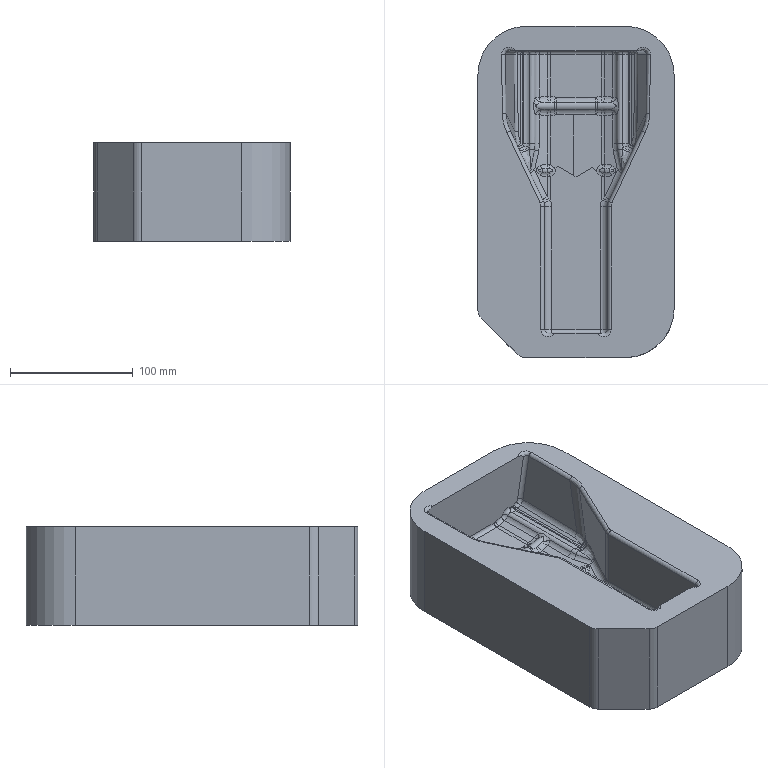NC program | NX | posted with a generic post | part box 160 x 270 x 80 mm
Lines 1 to 1083 of 159324:
N10 G17 G21 G94 G90
(CAVITY_MILL , TOOL : D25R5)
N12 T00 M6
N14 G54
N16 G17 G0 G90 X-4.895 Y47.373 S1200 M3
N18 G43 Z10. H0
N20 Z3.
N22 G94 G3 X5.06 Y53.831 Z-0.349 R11.25 F2000.
N24 G1 X10.121 Y64.585
N26 X-10.121
N28 X0. Y43.077
N30 X5.06 Y53.831
N32 X11.847 Y50.638
N34 X18.788 Y65.388
N36 X18.876 Y72.085
N38 X-18.876
N40 X-18.788 Y65.388
N42 X0. Y25.462
N44 X11.847 Y50.638
N46 X18.633 Y47.444
N48 X25.857 Y62.796
N50 G3 X26.278 Y64.583 R4.349
N52 G1 X26.476 Y79.585
N54 X-26.476
N56 X-26.278 Y64.583
N58 G3 X-25.852 Y62.787 R4.349
N60 G1 X0. Y7.848
N62 X18.633 Y47.444
N64 X25.419 Y44.251
N66 X32.639 Y59.595
N68 G3 X33.777 Y64.468 R11.849
N70 G1 X34.076 Y87.085
N72 X-34.076
N74 X-33.777 Y64.468
N76 G3 X-32.633 Y59.582 R11.849
N78 G1 X-5.628 Y2.194
N80 G2 X-2.469 Y-11.942 R33.204
N82 G1 Y-87.086
N84 X2.469
N86 Y-11.942
N88 G2 X5.628 Y2.194 R33.204
N90 G1 X25.419 Y44.251
N92 X32.205 Y41.058
N94 X39.419 Y56.387
N96 G3 X41.276 Y64.358 R19.349
N98 G1 X41.676 Y94.585
N100 X-41.676
N102 X-41.276 Y64.358
N104 G3 X-39.415 Y56.379 R19.349
N106 G1 X-12.415 Y-0.999
N108 G2 X-9.969 Y-11.942 R25.704
N110 G1 Y-94.587
N112 X9.969 Y-94.585
N114 Y-11.942
N116 G2 X12.415 Y-0.999 R25.704
N118 G1 X32.205 Y41.058
N120 X38.991 Y37.864
N122 X46.198 Y53.179
N124 G3 X48.775 Y64.25 R26.849
N126 G1 X49.309 Y104.589
N128 X49.247
N130 X49.191
N132 Y104.55
N134 X47.872 Y103.604
N136 X47.332 Y103.228
N138 X47.06 Y103.046
N140 X46.479 Y102.68
N142 X46.167 Y102.501
N144 X45.993 Y102.408
N146 X45.763 Y102.296
N148 X45.227 Y102.108
N150 X45.083 Y102.087
N152 X44.99 Y102.085
N154 X-44.954
N156 X-45.063 Y102.086
N158 X-45.2 Y102.103
N160 X-45.801 Y102.314
N162 X-46.028 Y102.426
N164 X-46.229 Y102.535
N166 X-46.478 Y102.68
N168 X-47.059 Y103.046
N170 X-48.197 Y103.837
N172 X-49.195 Y104.571
N174 Y104.589
N176 X-49.256
N178 X-49.309
N180 X-48.775 Y64.25
N182 G3 X-46.198 Y53.179 R26.849
N184 G1 X-19.201 Y-4.192
N186 G2 X-17.469 Y-11.942 R18.204
N188 G1 Y-104.589
N190 X-17.372
N192 X-16.937 Y-104.259
N194 X-15.66 Y-103.33
N196 X-15.469 Y-103.199
N198 X-15.241 Y-103.046
N200 X-14.694 Y-102.697
N202 X-14.143 Y-102.387
N204 X-13.757 Y-102.212
N206 X-13.432 Y-102.087
N208 X13.319 Y-102.085
N210 X13.515 Y-102.13
N212 X13.759 Y-102.213
N214 X13.961 Y-102.299
N216 X14.929 Y-102.843
N218 X15.241 Y-103.046
N220 X15.469 Y-103.199
N222 X17.19 Y-104.451
N224 X17.367 Y-104.589
N226 X17.469
N228 Y-11.942
N230 G2 X19.201 Y-4.192 R18.204
N232 G1 X38.991 Y37.864
N234 X27.681 Y43.187
N236 Z2.651
N238 G0 Z10.
N240 X-5.254 Y48.135
N242 Z2.651
N244 G3 X4.702 Y54.592 Z-0.699 R11.25
N246 G1 X9.404 Y64.585
N248 X-9.404
N250 X0. Y44.6
N252 X4.702 Y54.592
N254 X11.488 Y51.399
N256 X18.141 Y65.537
N258 X18.228 Y72.085
N260 X-18.228
N262 X-18.141 Y65.537
N264 X0. Y26.985
N266 X11.488 Y51.399
N268 X18.275 Y48.206
N270 X25.263 Y63.057
N272 G3 X25.63 Y64.621 R3.797
N274 G1 X25.828 Y79.585
N276 X-25.828
N278 X-25.63 Y64.646
N280 G3 X-25.257 Y63.044 R3.881
N282 G1 X0. Y9.37
N284 X18.275 Y48.206
N286 X25.061 Y45.012
N288 X32.047 Y59.858
N290 G3 X33.129 Y64.512 R11.297
N292 G1 X33.427 Y87.085
N294 X-33.427
N296 X-33.129 Y64.542
N298 G3 X-32.041 Y59.847 R11.381
N300 G1 X-5.045 Y2.478
N302 G2 X-1.821 Y-11.942 R33.852
N304 G1 Y-87.086
N306 X1.821
N308 Y-11.942
N310 G2 X5.036 Y2.457 R33.852
N312 G1 X25.061 Y45.012
N314 X31.847 Y41.819
N316 X38.827 Y56.653
N318 G3 X40.628 Y64.405 R18.797
N320 G1 X41.027 Y94.585
N322 X-41.027
N324 X-40.629 Y64.439
N326 G3 X-38.826 Y56.651 R18.881
N328 G1 X-11.831 Y-0.717
N330 G2 X-9.321 Y-11.942 R26.352
N332 G1 Y-94.587
N334 X9.321 Y-94.585
N336 Y-11.942
N338 G2 X11.823 Y-0.733 R26.352
N340 G1 X31.847 Y41.819
N342 X38.633 Y38.626
N344 X45.611 Y53.455
N346 G3 X48.127 Y64.3 R26.297
N348 G1 X48.654 Y104.097
N350 X48.56
N352 X47.872 Y103.604
N354 X47.332 Y103.228
N356 X47.06 Y103.046
N358 X46.479 Y102.68
N360 X46.167 Y102.501
N362 X45.993 Y102.408
N364 X45.763 Y102.296
N366 X45.227 Y102.108
N368 X45.083 Y102.087
N370 X44.99 Y102.085
N372 X-44.954
N374 X-45.063 Y102.086
N376 X-45.2 Y102.103
N378 X-45.801 Y102.314
N380 X-46.028 Y102.426
N382 X-46.229 Y102.535
N384 X-46.478 Y102.68
N386 X-47.059 Y103.046
N388 X-48.197 Y103.837
N390 X-48.551 Y104.097
N392 X-48.654
N394 X-48.128 Y64.336
N396 G3 X-45.611 Y53.455 R26.381
N398 G1 X-18.618 Y-3.908
N400 G2 X-16.821 Y-11.942 R18.852
N402 G1 Y-104.097
N404 X-16.714
N406 X-15.66 Y-103.33
N408 X-15.469 Y-103.199
N410 X-15.241 Y-103.046
N412 X-14.694 Y-102.697
N414 X-14.143 Y-102.387
N416 X-13.757 Y-102.212
N418 X-13.432 Y-102.087
N420 X13.319 Y-102.085
N422 X13.515 Y-102.13
N424 X13.759 Y-102.213
N426 X13.961 Y-102.299
N428 X14.929 Y-102.843
N430 X15.241 Y-103.046
N432 X15.469 Y-103.199
N434 X16.704 Y-104.097
N436 X16.821
N438 Y-11.942
N440 G2 X18.61 Y-3.926 R18.852
N442 G1 X38.633 Y38.626
N444 X27.323 Y43.948
N446 Z2.301
N448 G0 Z10.
N450 X-5.551 Y48.767
N452 Z2.301
N454 G3 X4.404 Y55.225 Z-1.048 R11.25
N456 G1 X8.809 Y64.585
N458 X-8.809
N460 X0. Y45.865
N462 X4.404 Y55.225
N464 X11.191 Y52.032
N466 X17.604 Y65.661
N468 X17.689 Y72.085
N470 X-17.689
N472 X-17.604 Y65.661
N474 X0. Y28.25
N476 X11.191 Y52.032
N478 X17.977 Y48.838
N480 X24.773 Y63.282
N482 G3 X25.091 Y64.611 R3.232
N484 G1 X25.289 Y79.585
N486 X-25.289
N488 X-25.091 Y64.644
N490 G3 X-24.753 Y63.239 R3.397
N492 G1 X0. Y10.636
N494 X17.977 Y48.838
N496 X24.763 Y45.645
N498 X31.554 Y60.077
N500 G3 X32.59 Y64.49 R10.732
N502 G1 X32.889 Y87.085
N504 X-32.889
N506 X-32.59 Y64.522
N508 G3 X-31.531 Y60.029 R10.897
N510 G1 X-4.558 Y2.706
N512 G2 X-1.282 Y-11.942 R34.391
N514 G1 Y-87.086
N516 X1.282
N518 Y-11.942
N520 G2 X4.545 Y2.679 R34.391
N522 G1 X24.763 Y45.645
N524 X31.549 Y42.452
N526 X38.329 Y56.86
N528 G3 X40.089 Y64.376 R18.232
N530 G1 X40.488 Y94.585
N532 X-40.488
N534 X-40.089 Y64.407
N536 G3 X-38.312 Y56.823 R18.397
N538 G1 X-11.343 Y-0.488
N540 G2 X-8.782 Y-11.942 R26.891
N542 G1 Y-94.586
N544 X8.782 Y-94.585
N546 Y-11.942
N548 G2 X11.333 Y-0.509 R26.891
N550 G1 X31.549 Y42.452
N552 X38.335 Y39.258
N554 X45.111 Y53.657
N556 G3 X47.588 Y64.265 R25.732
N558 G1 X48.11 Y103.7
N560 X48.006
N562 X47.872 Y103.604
N564 X47.332 Y103.228
N566 X47.06 Y103.046
N568 X46.479 Y102.68
N570 X46.167 Y102.501
N572 X45.993 Y102.408
N574 X45.763 Y102.296
N576 X45.227 Y102.108
N578 X45.083 Y102.087
N580 X44.99 Y102.085
N582 X-44.954
N584 X-45.063 Y102.086
N586 X-45.2 Y102.103
N588 X-45.801 Y102.314
N590 X-46.028 Y102.426
N592 X-46.229 Y102.535
N594 X-46.478 Y102.68
N596 X-47.059 Y103.046
N598 X-48. Y103.7
N600 X-48.11
N602 X-47.588 Y64.295
N604 G3 X-45.093 Y53.619 R25.897
N606 G1 X-18.13 Y-3.679
N608 G2 X-16.282 Y-11.942 R19.391
N610 G1 Y-103.7
N612 X-16.168
N614 X-15.66 Y-103.33
N616 X-15.469 Y-103.199
N618 X-15.241 Y-103.046
N620 X-14.694 Y-102.697
N622 X-14.143 Y-102.387
N624 X-13.757 Y-102.212
N626 X-13.432 Y-102.087
N628 X13.319 Y-102.085
N630 X13.515 Y-102.13
N632 X13.759 Y-102.213
N634 X13.961 Y-102.299
N636 X14.929 Y-102.843
N638 X15.241 Y-103.046
N640 X15.469 Y-103.199
N642 X16.157 Y-103.7
N644 X16.282
N646 Y-11.942
N648 G2 X18.12 Y-3.703 R19.391
N650 G1 X38.335 Y39.258
N652 X27.025 Y44.581
N654 Z1.952
N656 G0 Z10.
N658 X-5.807 Y49.31
N660 Z1.952
N662 G3 X4.149 Y55.768 Z-1.397 R11.25
N664 G1 X8.298 Y64.585
N666 X-8.298
N668 X0. Y46.951
N670 X4.149 Y55.768
N672 X10.935 Y52.575
N674 X17.143 Y65.767
N676 X17.227 Y72.085
N678 X-17.227
N680 X-17.143 Y65.767
N682 X0. Y29.336
N684 X10.935 Y52.575
N686 X17.721 Y49.381
N688 X24.325 Y63.415
N690 G3 X24.629 Y64.669 R3.03
N692 G1 X24.826 Y79.585
N694 X-24.826
N696 X-24.63 Y64.701
N698 G3 X-24.319 Y63.403 R3.14
N700 G1 X0. Y11.721
N702 X17.721 Y49.381
N704 X24.508 Y46.188
N706 X31.102 Y60.202
N708 G3 X32.128 Y64.544 R10.53
N710 G1 X32.426 Y87.085
N712 X-32.426
N714 X-32.129 Y64.583
N716 G3 X-31.099 Y60.195 R10.64
N718 G1 X-4.139 Y2.903
N720 G2 X-0.82 Y-11.942 R34.853
N722 G1 Y-87.086
N724 X0.82
N726 Y-11.942
N728 G2 X4.144 Y2.913 R34.853
N730 G1 X24.508 Y46.188
N732 X31.294 Y42.995
N734 X37.882 Y56.995
N736 G3 X39.627 Y64.427 R18.03
N738 G1 X40.026 Y94.585
N740 X-40.026
N742 X-39.628 Y64.471
N744 G3 X-37.88 Y56.992 R18.14
N746 G1 X-10.925 Y-0.292
N748 G2 X-8.32 Y-11.942 R27.353
N750 G1 Y-94.586
N752 X8.32 Y-94.585
N754 Y-11.942
N756 G2 X10.929 Y-0.282 R27.353
N758 G1 X31.294 Y42.995
N760 X38.08 Y39.801
N762 X44.663 Y53.79
N764 G3 X47.126 Y64.314 R25.53
N766 G1 X47.643 Y103.369
N768 X47.535
N770 X47.332 Y103.228
N772 X47.06 Y103.046
N774 X46.479 Y102.68
N776 X46.167 Y102.501
N778 X45.993 Y102.408
N780 X45.763 Y102.296
N782 X45.227 Y102.108
N784 X45.083 Y102.087
N786 X44.99 Y102.085
N788 X-44.954
N790 X-45.063 Y102.086
N792 X-45.2 Y102.103
N794 X-45.801 Y102.314
N796 X-46.028 Y102.426
N798 X-46.229 Y102.535
N800 X-46.478 Y102.68
N802 X-47.059 Y103.046
N804 X-47.524 Y103.369
N806 X-47.643
N808 X-47.127 Y64.362
N810 G3 X-44.663 Y53.79 R25.64
N812 G1 X-17.712 Y-3.483
N814 G2 X-15.82 Y-11.942 R19.853
N816 G1 Y-103.369
N818 X-15.713
N820 X-15.66 Y-103.33
N822 X-15.469 Y-103.199
N824 X-15.241 Y-103.046
N826 X-14.694 Y-102.697
N828 X-14.143 Y-102.387
N830 X-13.757 Y-102.212
N832 X-13.432 Y-102.087
N834 X13.319 Y-102.085
N836 X13.515 Y-102.13
N838 X13.759 Y-102.213
N840 X13.961 Y-102.299
N842 X14.929 Y-102.843
N844 X15.241 Y-103.046
N846 X15.469 Y-103.199
N848 X15.703 Y-103.369
N850 X15.82
N852 Y-11.942
N854 G2 X17.716 Y-3.475 R19.853
N856 G1 X38.08 Y39.801
N858 X26.77 Y45.123
N860 Z1.603
N862 G0 Z10.
N864 X-6.03 Y49.785
N866 Z1.603
N868 G3 X3.926 Y56.243 Z-1.747 R11.25
N870 G1 X7.851 Y64.585
N872 X-7.851
N874 X0. Y47.9
N876 X3.926 Y56.243
N878 X10.712 Y53.049
N880 X16.74 Y65.86
N882 X16.822 Y72.085
N884 X-16.822
N886 X-16.74 Y65.86
N888 X0. Y30.286
N890 X10.712 Y53.049
N892 X17.498 Y49.856
N894 X24. Y63.673
N896 G3 X24.224 Y64.615 R2.295
N898 G1 X24.422 Y79.585
N900 X-24.422
N902 X-24.224 Y64.615
N904 G3 X-23.996 Y63.665 R2.295
N906 G1 X0. Y12.671
N908 X17.498 Y49.856
N910 X24.284 Y46.663
N912 X30.782 Y60.472
N914 G3 X31.723 Y64.497 R9.795
N916 G1 X32.022 Y87.085
N918 X-32.022
N920 X-31.723 Y64.497
N922 G3 X-30.776 Y60.458 R9.795
N924 G1 X-3.773 Y3.074
N926 G2 X-0.416 Y-11.942 R35.257
N928 G1 Y-87.086
N930 X0.416
N932 Y-11.942
N934 G2 X3.774 Y3.077 R35.257
N936 G1 X24.284 Y46.663
N938 X31.07 Y43.469
N940 X37.561 Y57.262
N942 G3 X39.222 Y64.386 R17.295
N944 G1 X39.622 Y94.585
N946 X-39.622
N948 X-39.222 Y64.386
N950 G3 X-37.557 Y57.254 R17.295
N952 G1 X-10.559 Y-0.12
N954 G2 X-7.916 Y-11.942 R27.757
N956 G1 Y-94.586
N958 X7.916 Y-94.585
N960 Y-11.942
N962 G2 X10.56 Y-0.117 R27.757
N964 G1 X31.07 Y43.469
N966 X37.857 Y40.276
N968 X44.34 Y54.053
N970 G3 X46.722 Y64.277 R24.795
N972 G1 X47.235 Y103.09
N974 X47.126
N976 X47.06 Y103.046
N978 X46.479 Y102.68
N980 X46.167 Y102.501
N982 X45.993 Y102.408
N984 X45.763 Y102.296
N986 X45.227 Y102.108
N988 X45.083 Y102.087
N990 X44.99 Y102.085
N992 X-44.954
N994 X-45.063 Y102.086
N996 X-45.2 Y102.103
N998 X-45.801 Y102.314
N1000 X-46.028 Y102.426
N1002 X-46.229 Y102.535
N1004 X-46.478 Y102.68
N1006 X-47.059 Y103.046
N1008 X-47.123 Y103.09
N1010 X-47.235
N1012 X-46.722 Y64.277
N1014 G3 X-44.34 Y54.053 R24.795
N1016 G1 X-17.346 Y-3.312
N1018 G2 X-15.416 Y-11.942 R20.257
N1020 G1 Y-103.09
N1022 X-15.307
N1024 X-15.241 Y-103.046
N1026 X-14.694 Y-102.697
N1028 X-14.143 Y-102.387
N1030 X-13.757 Y-102.212
N1032 X-13.432 Y-102.087
N1034 X13.319 Y-102.085
N1036 X13.515 Y-102.13
N1038 X13.759 Y-102.213
N1040 X13.961 Y-102.299
N1042 X14.929 Y-102.843
N1044 X15.241 Y-103.046
N1046 X15.307 Y-103.09
N1048 X15.416
N1050 Y-11.942
N1052 G2 X17.348 Y-3.307 R20.257
N1054 G1 X37.857 Y40.276
N1056 X26.546 Y45.598
N1058 Z1.253
N1060 G0 Z10.
N1062 X-6.228 Y50.205
N1064 Z1.253
N1066 G3 X3.728 Y56.663 Z-2.096 R11.25
N1068 G1 X7.456 Y64.585
N1070 X-7.456
N1072 X0. Y48.74
N1074 X3.728 Y56.663
N1076 X10.514 Y53.469
N1078 X16.383 Y65.942
N1080 X16.465 Y72.085
N1082 X-16.465
N1084 X-16.383 Y65.942
N1086 X0. Y31.126
N1088 X10.514 Y53.469
N1090 X17.3 Y50.276
N1092 X23.641 Y63.75
N1094 G3 X23.867 Y64.678 R2.257
N1096 G1 X24.064 Y79.585
N1098 X-24.064
N1100 X-23.868 Y64.719
N1102 G3 X-23.628 Y63.723 R2.404
N1104 G1 X0. Y13.511
N1106 X17.3 Y50.276
N1108 X24.087 Y47.083
N1110 X30.419 Y60.54
N1112 G3 X31.366 Y64.547 R9.757
N1114 G1 X31.664 Y87.085
N1116 X-31.664
N1118 X-31.367 Y64.598
N1120 G3 X-30.407 Y60.514 R9.904
N1122 G1 X-3.449 Y3.225
N1124 G2 X-0.058 Y-11.942 R35.615
N1126 G1 Y-87.086
N1128 X0.058
N1130 Y-11.942
N1132 G2 X3.442 Y3.211 R35.615
N1134 G1 X24.087 Y47.083
N1136 X30.873 Y43.889
N1138 X37.19 Y57.314
N1140 G3 X38.865 Y64.427 R17.257
N1142 G1 X39.264 Y94.585
N1144 X-39.264
N1146 X-38.866 Y64.486
N1148 G3 X-37.188 Y57.31 R17.404
N1150 G1 X-10.235 Y0.031
N1152 G2 X-7.558 Y-11.942 R28.115
N1154 G1 Y-94.586
N1156 X7.558 Y-94.585
N1158 Y-11.942
N1160 G2 X10.229 Y0.02 R28.115
N1162 G1 X30.873 Y43.889
N1164 X37.659 Y40.696
N1166 X43.97 Y54.108
N1168 G3 X46.364 Y64.312 R24.757
N1170 G1 X46.874 Y102.854
N1172 X46.755
N1174 X46.479 Y102.68
N1176 X46.167 Y102.501
N1178 X45.993 Y102.408
N1180 X45.763 Y102.296
N1182 X45.227 Y102.108
N1184 X45.083 Y102.087
N1186 X44.99 Y102.085
N1188 X-44.954
N1190 X-45.063 Y102.086
N1192 X-45.2 Y102.103
N1194 X-45.801 Y102.314
N1196 X-46.028 Y102.426
N1198 X-46.229 Y102.535
N1200 X-46.478 Y102.68
N1202 X-46.755 Y102.854
N1204 X-46.874
N1206 X-46.365 Y64.375
N1208 G3 X-43.97 Y54.108 R24.904
N1210 G1 X-17.021 Y-3.162
N1212 G2 X-15.058 Y-11.942 R20.615
N1214 G1 Y-102.854
N1216 X-14.94
N1218 X-14.694 Y-102.697
N1220 X-14.143 Y-102.387
N1222 X-13.757 Y-102.212
N1224 X-13.432 Y-102.087
N1226 X13.319 Y-102.085
N1228 X13.515 Y-102.13
N1230 X13.759 Y-102.213
N1232 X13.961 Y-102.299
N1234 X14.929 Y-102.843
N1236 X14.946 Y-102.854
N1238 X15.058
N1240 Y-11.942
N1242 G2 X17.016 Y-3.173 R20.615
N1244 G1 X37.659 Y40.696
N1246 X26.349 Y46.018
N1248 Z0.904
N1250 G0 Z10.
N1252 X-6.404 Y50.58
N1254 Z0.904
N1256 G3 X3.552 Y57.037 Z-2.446 R11.25
N1258 G1 X7.103 Y64.585
N1260 X-7.103
N1262 X0. Y49.49
N1264 X3.552 Y57.037
N1266 X10.338 Y53.844
N1268 X16.065 Y66.015
N1270 X16.146 Y72.085
N1272 X-16.146
N1274 X-16.065 Y66.015
N1276 X0. Y31.875
N1278 X10.338 Y53.844
N1280 X17.124 Y50.651
N1282 X23.354 Y63.89
N1284 G3 X23.548 Y64.697 R2.004
N1286 G1 X23.745 Y79.585
N1288 X-23.745
N1290 X-23.549 Y64.723
N1292 G3 X-23.336 Y63.852 R2.096
N1294 G1 X0. Y14.26
N1296 X17.124 Y50.651
N1298 X23.91 Y47.457
N1300 X30.125 Y60.663
N1302 G3 X31.047 Y64.565 R9.504
N1304 G1 X31.345 Y87.085
N1306 X-31.345
N1308 X-31.048 Y64.597
N1310 G3 X-30.114 Y60.64 R9.596
N1312 G1 X-3.155 Y3.349
N1314 G2 X0. Y-7.618 R35.934
N1316 X3.148 Y3.334 R35.934
N1318 G1 X23.91 Y47.457
N1320 X30.696 Y44.264
N1322 X36.895 Y57.436
N1324 G3 X38.546 Y64.445 R17.004
N1326 G1 X38.945 Y94.585
N1328 X-38.945
N1330 X-38.547 Y64.481
N1332 G3 X-36.894 Y57.433 R17.096
N1334 G1 X-9.942 Y0.158
N1336 G2 X-7.239 Y-11.942 R28.434
N1338 G1 Y-94.586
N1340 X7.239 Y-94.585
N1342 Y-11.942
N1344 G2 X9.936 Y0.146 R28.434
N1346 G1 X30.696 Y44.264
N1348 X37.483 Y41.071
N1350 X43.675 Y54.229
N1352 G3 X46.046 Y64.329 R24.504
N1354 G1 X46.553 Y102.654
N1356 X46.434
N1358 X46.167 Y102.501
N1360 X45.993 Y102.408
N1362 X45.763 Y102.296
N1364 X45.227 Y102.108
N1366 X45.083 Y102.087
N1368 X44.99 Y102.085
N1370 X-44.954
N1372 X-45.063 Y102.086
N1374 X-45.2 Y102.103
N1376 X-45.801 Y102.314
N1378 X-46.028 Y102.426
N1380 X-46.229 Y102.535
N1382 X-46.434 Y102.654
N1384 X-46.553
N1386 X-46.046 Y64.369
N1388 G3 X-43.675 Y54.229 R24.596
N1390 G1 X-16.73 Y-3.032
N1392 G2 X-14.739 Y-11.942 R20.934
N1394 G1 Y-102.654
N1396 X-14.618
N1398 X-14.143 Y-102.387
N1400 X-13.757 Y-102.212
N1402 X-13.432 Y-102.087
N1404 X13.319 Y-102.085
N1406 X13.515 Y-102.13
N1408 X13.759 Y-102.213
N1410 X13.961 Y-102.299
N1412 X14.593 Y-102.654
N1414 X14.739
N1416 Y-11.942
N1418 G2 X16.722 Y-3.047 R20.934
N1420 G1 X37.483 Y41.071
N1422 X26.172 Y46.393
N1424 Z0.554
N1426 G0 Z10.
N1428 X-6.562 Y50.915
N1430 Z0.554
N1432 G3 X3.394 Y57.373 Z-2.795 R11.25
N1434 G1 X6.788 Y64.585
N1436 X-6.787
N1438 X0. Y50.161
N1440 X3.394 Y57.373
N1442 X10.18 Y54.18
N1444 X15.78 Y66.081
N1446 X15.86 Y72.085
N1448 X-15.86
N1450 X-15.78 Y66.081
N1452 X0. Y32.546
N1454 X10.18 Y54.18
N1456 X16.966 Y50.986
N1458 X23.101 Y64.024
N1460 G3 X23.263 Y64.7 R1.677
N1462 G1 X23.46 Y79.585
N1464 X-23.46
N1466 X-23.263 Y64.729
N1468 G3 X-23.1 Y64.021 R1.717
N1470 G1 X0. Y14.931
N1472 X16.966 Y50.986
N1474 X23.752 Y47.793
N1476 X29.877 Y60.808
N1478 G3 X30.762 Y64.573 R9.177
N1480 G1 X31.059 Y87.085
N1482 X-31.059
N1484 X-30.762 Y64.63
N1486 G3 X-29.886 Y60.828 R9.217
N1488 G1 X-2.89 Y3.458
N1490 G2 X0. Y-5.671 R36.22
N1492 X2.903 Y3.485 R36.22
N1494 G1 X23.752 Y47.793
N1496 X30.539 Y44.599
N1498 X36.653 Y57.593
N1500 G3 X38.261 Y64.457 R16.677
N1502 G1 X38.659 Y94.585
N1504 X-38.659
N1506 X-38.262 Y64.531
N1508 G3 X-36.672 Y57.634 R16.717
N1510 G1 X-9.678 Y0.27
N1512 G2 X-6.953 Y-11.942 R28.72
N1514 G1 Y-94.586
N1516 X6.953 Y-94.585
N1518 Y-11.942
N1520 G2 X9.689 Y0.292 R28.72
N1522 G1 X30.539 Y44.599
N1524 X37.325 Y41.406
N1526 X43.428 Y54.377
N1528 G3 X45.76 Y64.344 R24.177
N1530 G1 X46.264 Y102.486
N1532 X46.14
N1534 X45.993 Y102.408
N1536 X45.763 Y102.296
N1538 X45.227 Y102.108
N1540 X45.083 Y102.087
N1542 X44.99 Y102.085
N1544 X-44.954
N1546 X-45.063 Y102.086
N1548 X-45.2 Y102.103
N1550 X-45.801 Y102.314
N1552 X-46.028 Y102.426
N1554 X-46.139 Y102.486
N1556 X-46.264
N1558 X-45.761 Y64.432
N1560 G3 X-43.458 Y54.441 R24.217
N1562 G1 X-16.469 Y-2.915
N1564 G2 X-14.453 Y-11.942 R21.22
N1566 G1 Y-102.486
N1568 X-14.319
N1570 X-14.143 Y-102.387
N1572 X-13.757 Y-102.212
N1574 X-13.432 Y-102.087
N1576 X13.319 Y-102.085
N1578 X13.515 Y-102.13
N1580 X13.759 Y-102.213
N1582 X13.961 Y-102.299
N1584 X14.294 Y-102.486
N1586 X14.453
N1588 Y-11.942
N1590 G2 X16.476 Y-2.9 R21.22
N1592 G1 X37.325 Y41.406
N1594 X26.014 Y46.728
N1596 Z0.205
N1598 G0 Z10.
N1600 X10.082 Y58.326
N1602 Z0.205
N1604 G3 X0. Y64.585 Z-3.144 R11.25
N1606 G1 X-6.504
N1608 X0. Y50.763
N1610 X6.504 Y64.585
N1612 X0.
N1614 Y72.085
N1616 X-15.603
N1618 X-15.524 Y66.14
N1620 X0. Y33.149
N1622 X15.524 Y66.139
N1624 X15.603 Y72.085
N1626 X0.
N1628 Y79.585
N1630 X-23.203
N1632 X-23.006 Y64.677
N1634 G3 X-22.862 Y64.119 R1.324
N1636 G1 X0. Y15.534
N1638 X22.878 Y64.151
N1640 G3 X23.006 Y64.677 R1.324
N1642 G1 X23.203 Y79.585
N1644 X0.
N1646 Y87.085
N1648 X-30.803
N1650 X-30.505 Y64.535
N1652 G3 X-29.635 Y60.898 R8.824
N1654 G1 X-2.661 Y3.573
N1656 G2 X0. Y-4.328 R36.476
N1658 X2.667 Y3.588 R36.476
N1660 G1 X29.649 Y60.926
N1662 G3 X30.505 Y64.535 R8.824
N1664 G1 X30.803 Y87.085
N1666 X0.
N1668 Y94.585
N1670 X-38.403
N1672 X-38.004 Y64.411
N1674 G3 X-36.412 Y57.684 R16.324
N1676 G1 X-9.448 Y0.383
N1678 X-9.442 Y0.37
N1680 G2 X-6.697 Y-11.942 R28.976
N1682 G1 Y-94.586
N1684 X6.697 Y-94.585
N1686 Y-11.942
N1688 G2 X9.454 Y0.395 R28.976
N1690 G1 X36.42 Y57.7
N1692 G3 X38.004 Y64.411 R16.324
N1694 G1 X38.403 Y94.585
N1696 X0.
N1698 Y102.085
N1700 X-44.954
N1702 X-45.063 Y102.086
N1704 X-45.2 Y102.103
N1706 X-45.801 Y102.314
N1708 X-45.869 Y102.348
N1710 X-46.006
N1712 X-45.503 Y64.293
N1714 G3 X-43.191 Y54.475 R23.824
N1716 G1 X-16.235 Y-2.81
N1718 G2 X-14.197 Y-11.942 R21.476
N1720 G1 Y-102.348
N1722 X-14.055
N1724 X-13.757 Y-102.212
N1726 X-13.432 Y-102.087
N1728 X13.319 Y-102.085
N1730 X13.515 Y-102.13
N1732 X13.759 Y-102.213
N1734 X13.961 Y-102.299
N1736 X14.047 Y-102.348
N1738 X14.197
N1740 Y-11.942
N1742 G2 X16.24 Y-2.798 R21.476
N1744 G1 X43.191 Y54.475
N1746 G3 X45.503 Y64.293 R23.824
N1748 G1 X46.006 Y102.348
N1750 X45.868
N1752 X45.763 Y102.296
N1754 X45.227 Y102.108
N1756 X45.083 Y102.087
N1758 X44.99 Y102.085
N1760 X0.
N1762 Y89.585
N1764 Z-0.144
N1766 G0 Z10.
N1768 X10.082 Y58.326
N1770 Z-0.144
N1772 G3 X0. Y64.585 Z-3.494 R11.25
N1774 G1 X-6.249
N1776 X0. Y51.305
N1778 X6.249 Y64.585
N1780 X0.
N1782 Y72.085
N1784 X-15.372
N1786 X-15.295 Y66.193
N1788 X0. Y33.69
N1790 X15.295 Y66.193
N1792 X15.372 Y72.085
N1794 X0.
N1796 Y79.585
N1798 X-22.972
N1800 X-22.776 Y64.742
N1802 G3 X-22.635 Y64.178 R1.346
N1804 G1 X0. Y16.076
N1806 X22.675 Y64.261
N1808 G3 X22.775 Y64.673 R1.038
N1810 G1 X22.972 Y79.585
N1812 X0.
N1814 Y87.085
N1816 X-30.572
N1818 X-30.275 Y64.613
N1820 G3 X-29.412 Y60.965 R8.846
N1822 G1 X-2.47 Y3.709
N1824 G2 X0. Y-3.29 R36.707
N1826 X2.455 Y3.677 R36.707
N1828 G1 X29.444 Y61.032
N1830 G3 X30.274 Y64.534 R8.538
N1832 G1 X30.572 Y87.085
N1834 X0.
N1836 Y94.585
N1838 X-38.172
N1840 X-37.774 Y64.496
N1842 G3 X-36.192 Y57.757 R16.346
N1844 G1 X-9.257 Y0.518
N1846 X-9.253 Y0.51
N1848 G2 X-6.466 Y-11.942 R29.207
N1850 G1 Y-94.586
N1852 X6.466 Y-94.585
N1854 Y-11.942
N1856 G2 X9.242 Y0.486 R29.207
N1858 G1 X36.213 Y57.803
N1860 G3 X37.773 Y64.413 R16.038
N1862 G1 X38.172 Y94.585
N1864 X0.
N1866 Y102.085
N1868 X-44.954
N1870 X-45.063 Y102.086
N1872 X-45.2 Y102.103
N1874 X-45.577 Y102.235
N1876 X-45.774
N1878 X-45.273 Y64.382
N1880 G3 X-42.972 Y54.552 R23.846
N1882 G1 X-16.043 Y-2.676
N1884 G2 X-13.966 Y-11.942 R21.707
N1886 G1 Y-102.235
N1888 X-13.809
N1890 X-13.757 Y-102.212
N1892 X-13.432 Y-102.087
N1894 X13.319 Y-102.085
N1896 X13.515 Y-102.13
N1898 X13.759 Y-102.213
N1900 X13.812 Y-102.235
N1902 X13.966
N1904 Y-11.942
N1906 G2 X16.028 Y-2.707 R21.707
N1908 G1 X42.992 Y54.595
N1910 G3 X45.272 Y64.296 R23.538
N1912 G1 X45.774 Y102.235
N1914 X45.589
N1916 X45.227 Y102.108
N1918 X45.083 Y102.087
N1920 X44.99 Y102.085
N1922 X0.
N1924 Y89.585
N1926 Z-0.494
N1928 G0 Z10.
N1930 X10.082 Y58.326
N1932 Z-0.494
N1934 G3 X0. Y64.585 Z-3.843 R11.25
N1936 G1 X-6.02
N1938 X0. Y51.791
N1940 X6.02 Y64.585
N1942 X0.
N1944 Y72.085
N1946 X-15.165
N1948 X-15.088 Y66.241
N1950 X0. Y34.177
N1952 X15.088 Y66.241
N1954 X15.165 Y72.085
N1956 X0.
N1958 Y79.585
N1960 X-22.765
N1962 X-22.568 Y64.695
N1964 G3 X-22.49 Y64.356 R0.823
N1966 G1 X0. Y16.562
N1968 X22.495 Y64.367
N1970 G3 X22.568 Y64.683 R0.768
N1972 G1 X22.765 Y79.585
N1974 X0.
N1976 Y87.085
N1978 X-30.365
N1980 X-30.068 Y64.596
N1982 G3 X-29.276 Y61.162 R8.323
N1984 G1 X-2.284 Y3.8
N1986 G2 X0. Y-2.45 R36.914
N1988 X2.274 Y3.78 R36.914
N1990 G1 X29.281 Y61.173
N1992 G3 X30.068 Y64.584 R8.268
N1994 G1 X30.365 Y87.085
N1996 X0.
N1998 Y94.585
N2000 X-37.965
N2002 X-37.567 Y64.497
N2004 G3 X-36.063 Y57.969 R15.823
N2006 G1 X-9.069 Y0.604
N2008 G2 X-6.259 Y-11.942 R29.414
N2010 G1 Y-94.586
N2012 X6.259 Y-94.585
N2014 Y-11.942
N2016 G2 X9.06 Y0.587 R29.414
N2018 G1 X36.068 Y57.98
N2020 G3 X37.567 Y64.485 R15.768
N2022 G1 X37.965 Y94.585
N2024 X0.
N2026 Y102.085
N2028 X-44.954
N2030 X-45.063 Y102.086
N2032 X-45.2 Y102.103
N2034 X-45.329 Y102.148
N2036 X-45.566
N2038 X-45.066 Y64.398
N2040 G3 X-42.849 Y54.776 R23.323
N2042 G1 X-15.86 Y-2.578
N2044 G2 X-13.759 Y-11.942 R21.914
N2046 G1 Y-102.148
N2048 X-13.591
N2050 X-13.432 Y-102.087
N2052 X13.319 Y-102.085
N2054 X13.515 Y-102.13
N2056 X13.567 Y-102.148
N2058 X13.759
N2060 Y-11.942
N2062 G2 X15.848 Y-2.604 R21.914
N2064 G1 X42.854 Y54.786
N2066 G3 X45.066 Y64.386 R23.268
N2068 G1 X45.566 Y102.148
N2070 X45.341
N2072 X45.227 Y102.108
N2074 X45.083 Y102.087
N2076 X44.99 Y102.085
N2078 X0.
N2080 Y89.585
N2082 Z-0.843
N2084 G0 Z10.
N2086 X-7.048 Y51.948
N2088 Z-0.843
N2090 G3 X2.908 Y58.406 Z-4.192 R11.25
N2092 G1 X5.815 Y64.585
N2094 X-5.815
N2096 X0. Y52.227
N2098 X2.908 Y58.406
N2100 X9.694 Y55.212
N2102 X14.903 Y66.283
N2104 X14.98 Y72.085
N2106 X-14.98
N2108 X-14.903 Y66.283
N2110 X0. Y34.612
N2112 X9.694 Y55.212
N2114 X16.48 Y52.019
N2116 X22.32 Y64.429
N2118 G3 X22.383 Y64.704 R0.668
N2120 G1 X22.58 Y79.585
N2122 X-22.58
N2124 X-22.383 Y64.723
N2126 G3 X-22.312 Y64.412 R0.756
N2128 G1 X0. Y16.997
N2130 X16.48 Y52.019
N2132 X23.266 Y48.826
N2134 X29.106 Y61.235
N2136 G3 X29.882 Y64.605 R8.168
N2138 G1 X30.18 Y87.085
N2140 X-30.18
N2142 X-29.883 Y64.624
N2144 G3 X-29.098 Y61.218 R8.256
N2146 G1 X-2.085 Y3.814
N2148 G2 X0. Y-1.753 R37.099
N2150 X2.098 Y3.841 R37.099
N2152 G1 X23.266 Y48.826
N2154 X30.052 Y45.632
N2156 X35.892 Y58.042
N2158 G3 X37.382 Y64.506 R15.668
N2160 G1 X37.78 Y94.585
N2162 X-37.78
N2164 X-37.382 Y64.525